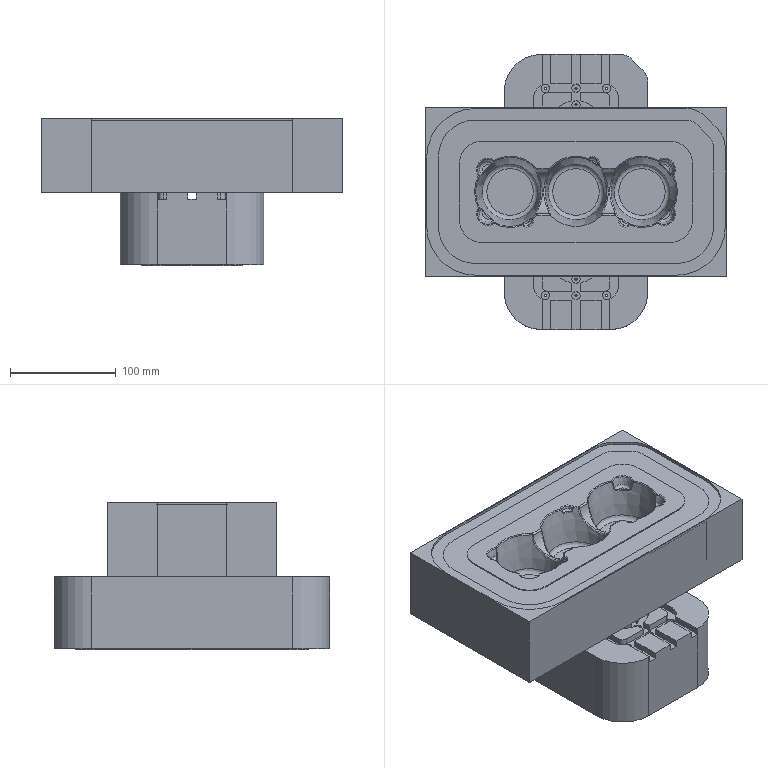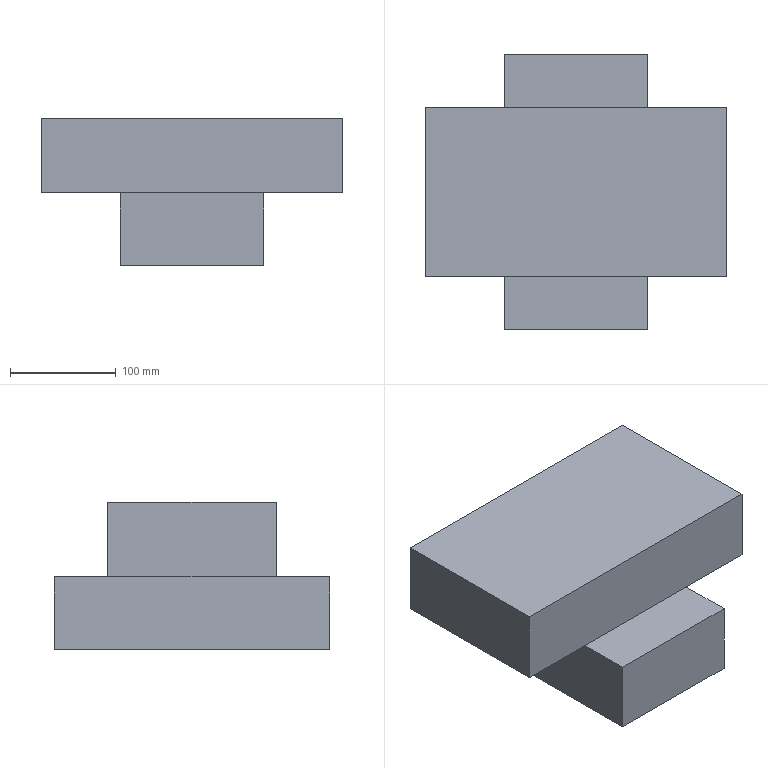CAM job | NX | 3-axis milling, drilling | part box 284.317 x 260.317 x 139.5 mm | stock box 284.317 x 260.317 x 139.5 mm
Tools:
number,name,description,diameter,corner_radius,flute_length,length,flutes
0,V2.0,Drilling Tool,2.0,0.0,35.0,50.0,2
0,V8.0,Drilling Tool,8.0,0.0,35.0,50.0,2
0,D10,No Description,10.0,0.0,20.0,60.0,2
0,D8,No Description,8.0,0.0,0.0,40.0,2
0,D16R0.8,No Description,16.0,0.8,50.0,90.0,2
0,R2,No Description,4.0,2.0,0.0,20.0,2
Operations:
program,operation,operation_type,tool,method,geometry_group,spindle_rpm,surface_speed,feed_per_tooth,feed_cut,feed_plunge,cut_length_mm,path_length_mm,cut_time_min,machine_time_min
B-1,B1,CavityMilling,D16R0.8,METHOD,22B,7000.0,1099.0,0.3214,4500.0,100.0,93028.313,99021.605,20.673,21.272
B-2,B5,SurfaceContour,R2,METHOD,22B,8000.0,251.0,0.2812,4500.0,100.0,125715.456,127167.179,27.937,28.082
B-2,B4,Engraving,R2,METHOD,22B,9000.0,113.0,0.1111,2000.0,100.0,642.356,8918.57,0.6703,1.498
B-3,DRILLING,Operation,V2.0,METHOD,22B,2000.0,75.0,0.0375,150.0,0.0,195.0,1865.363,1.3,1.467
B-4,B6,FaceMilling,D10,METHOD,22B,7000.0,1099.0,0.2857,4000.0,100.0,4167.722,4469.722,1.042,1.072
B-4,B7,PlanarMilling,D10,METHOD,22B,7000.0,571.0,0.2857,4000.0,100.0,79571.113,79941.883,19.893,19.93
C-1,CAVITY_MILL,CavityMilling,D8,METHOD,23C,7000.0,1099.0,0.3214,4500.0,100.0,66252.078,85679.087,14.723,16.665
C-2,DRILLING_1,Operation,V2.0,METHOD,23C,2000.0,75.0,0.0375,150.0,0.0,195.0,1645.678,1.3,1.445
C-3,DRILLING_1_COPY,Operation,V8.0,METHOD,23C,2000.0,75.0,0.0375,150.0,0.0,828.0,2503.865,5.52,5.688
C-3,DRILLING_1_COPY_COPY,Operation,V8.0,METHOD,23C,2000.0,75.0,0.0375,150.0,0.0,105.0,901.705,0.7,0.7797
C-3,DRILLING_1_COPY_COPY_1,Operation,V8.0,METHOD,23C,2000.0,75.0,0.0375,150.0,0.0,132.0,728.868,0.88,0.9397